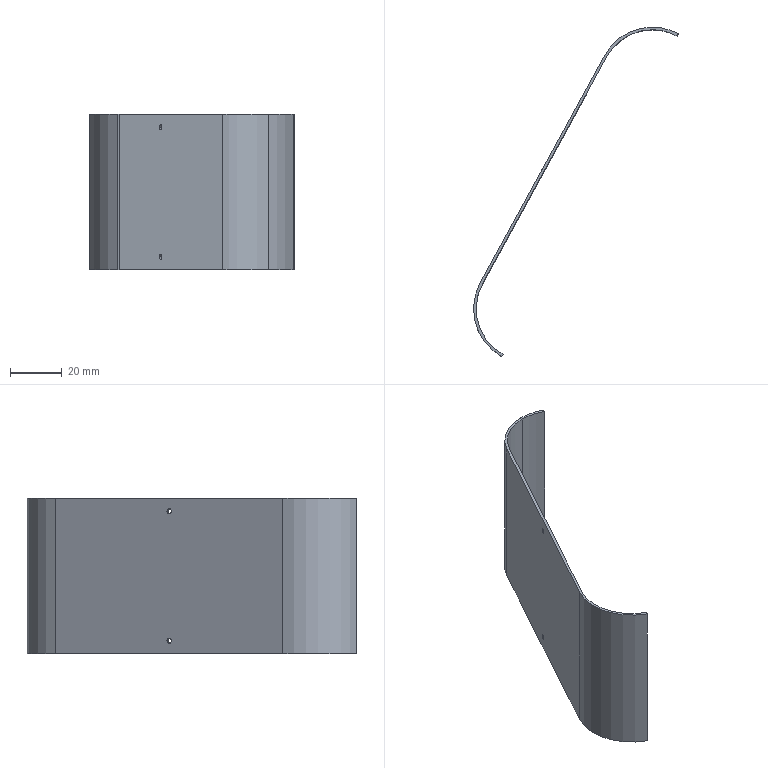Part | SolidWorks | features BaseBody 1 | 1 solid | 16 faces | box 79.069 x 127.155 x 60 mm | volume 9858 mm3 | cylinder 10 | plane 6 | commonest cylinder face diameters 2 x4 40 x3 42 x3
STEP:
#1=CARTESIAN_POINT('',(513.262,10.517,305.544));
#2=VERTEX_POINT('',#1);
#3=CARTESIAN_POINT('',(494.838,-0.4052,305.544));
#4=VERTEX_POINT('',#3);
#5=CARTESIAN_POINT('',(513.262,-10.483,305.544));
#6=DIRECTION('',(0.000000004,-0.000000009,1.));
#7=DIRECTION('',(0.,1.,0.000000009));
#8=AXIS2_PLACEMENT_3D('',#5,#6,#7);
#9=CIRCLE('',#8,21.);
#10=EDGE_CURVE('',#2,#4,#9,.T.);
#11=ORIENTED_EDGE('',*,*,#10,.F.);
#12=CARTESIAN_POINT('',(513.262,10.517,245.544));
#13=VERTEX_POINT('',#12);
#14=CARTESIAN_POINT('',(513.262,10.517,305.544));
#15=DIRECTION('',(-0.000000004,0.000000009,-1.));
#16=VECTOR('',#15,1000.);
#17=LINE('',#14,#16);
#18=EDGE_CURVE('',#2,#13,#17,.T.);
#19=ORIENTED_EDGE('',*,*,#18,.T.);
#20=CARTESIAN_POINT('',(494.838,-0.4052,245.544));
#21=VERTEX_POINT('',#20);
#22=CARTESIAN_POINT('',(513.262,-10.483,245.544));
#23=DIRECTION('',(-0.000000004,0.000000009,-1.));
#24=DIRECTION('',(0.,1.,0.000000009));
#25=AXIS2_PLACEMENT_3D('',#22,#23,#24);
#26=CIRCLE('',#25,21.);
#27=EDGE_CURVE('',#21,#13,#26,.T.);
#28=ORIENTED_EDGE('',*,*,#27,.F.);
#29=CARTESIAN_POINT('',(494.838,-0.4052,275.544));
#30=DIRECTION('',(-0.000000007,0.000000004,-1.));
#31=VECTOR('',#30,1000.);
#32=LINE('',#29,#31);
#33=EDGE_CURVE('',#4,#21,#32,.T.);
#34=ORIENTED_EDGE('',*,*,#33,.F.);
#35=EDGE_LOOP('',(#11,#19,#28,#34));
#36=FACE_OUTER_BOUND('',#35,.T.);
#37=CARTESIAN_POINT('',(513.262,-10.483,305.544));
#38=DIRECTION('',(-0.000000004,0.000000009,-1.));
#39=DIRECTION('',(0.,1.,0.000000009));
#40=AXIS2_PLACEMENT_3D('',#37,#38,#39);
#41=CYLINDRICAL_SURFACE('',#40,21.);
#42=ADVANCED_FACE('',(#36),#41,.T.);
#43=CARTESIAN_POINT('',(472.199,-43.874,300.544));
#44=VERTEX_POINT('',#43);
#45=CARTESIAN_POINT('',(471.24,-45.628,300.544));
#46=VERTEX_POINT('',#45);
#47=CARTESIAN_POINT('',(471.72,-44.751,300.544));
#48=DIRECTION('',(-0.8773,0.4799,0.000000008));
#49=DIRECTION('',(-0.4799,-0.8773,0.));
#50=AXIS2_PLACEMENT_3D('',#47,#48,#49);
#51=CIRCLE('',#50,1.);
#52=EDGE_CURVE('',#44,#46,#51,.T.);
#53=ORIENTED_EDGE('',*,*,#52,.F.);
#54=CARTESIAN_POINT('',(471.322,-43.394,300.544));
#55=VERTEX_POINT('',#54);
#56=CARTESIAN_POINT('',(471.313,-43.389,300.544));
#57=DIRECTION('',(-0.8773,0.4799,0.000000008));
#58=VECTOR('',#57,1000.);
#59=LINE('',#56,#58);
#60=EDGE_CURVE('',#44,#55,#59,.T.);
#61=ORIENTED_EDGE('',*,*,#60,.T.);
#62=CARTESIAN_POINT('',(470.362,-45.148,300.544));
#63=VERTEX_POINT('',#62);
#64=CARTESIAN_POINT('',(470.842,-44.271,300.544));
#65=DIRECTION('',(0.8773,-0.4799,-0.000000008));
#66=DIRECTION('',(-0.4799,-0.8773,0.));
#67=AXIS2_PLACEMENT_3D('',#64,#65,#66);
#68=CIRCLE('',#67,1.);
#69=EDGE_CURVE('',#63,#55,#68,.T.);
#70=ORIENTED_EDGE('',*,*,#69,.F.);
#71=CARTESIAN_POINT('',(470.354,-45.144,300.544));
#72=DIRECTION('',(-0.8773,0.4799,0.000000008));
#73=VECTOR('',#72,1000.);
#74=LINE('',#71,#73);
#75=EDGE_CURVE('',#46,#63,#74,.T.);
#76=ORIENTED_EDGE('',*,*,#75,.F.);
#77=EDGE_LOOP('',(#53,#61,#70,#76));
#78=FACE_OUTER_BOUND('',#77,.T.);
#79=CARTESIAN_POINT('',(470.833,-44.266,300.544));
#80=DIRECTION('',(-0.8773,0.4799,0.000000008));
#81=DIRECTION('',(-0.4799,-0.8773,0.));
#82=AXIS2_PLACEMENT_3D('',#79,#80,#81);
#83=CYLINDRICAL_SURFACE('',#82,1.);
#84=ADVANCED_FACE('',(#78),#83,.F.);
#85=CARTESIAN_POINT('',(472.199,-43.874,250.544));
#86=VERTEX_POINT('',#85);
#87=CARTESIAN_POINT('',(471.24,-45.628,250.544));
#88=VERTEX_POINT('',#87);
#89=CARTESIAN_POINT('',(471.72,-44.751,250.544));
#90=DIRECTION('',(-0.8773,0.4799,0.000000008));
#91=DIRECTION('',(-0.4799,-0.8773,0.));
#92=AXIS2_PLACEMENT_3D('',#89,#90,#91);
#93=CIRCLE('',#92,1.);
#94=EDGE_CURVE('',#86,#88,#93,.T.);
#95=ORIENTED_EDGE('',*,*,#94,.F.);
#96=CARTESIAN_POINT('',(471.322,-43.394,250.544));
#97=VERTEX_POINT('',#96);
#98=CARTESIAN_POINT('',(471.313,-43.389,250.544));
#99=DIRECTION('',(-0.8773,0.4799,0.000000008));
#100=VECTOR('',#99,1000.);
#101=LINE('',#98,#100);
#102=EDGE_CURVE('',#86,#97,#101,.T.);
#103=ORIENTED_EDGE('',*,*,#102,.T.);
#104=CARTESIAN_POINT('',(470.362,-45.148,250.544));
#105=VERTEX_POINT('',#104);
#106=CARTESIAN_POINT('',(470.842,-44.271,250.544));
#107=DIRECTION('',(0.8773,-0.4799,-0.000000008));
#108=DIRECTION('',(-0.4799,-0.8773,0.));
#109=AXIS2_PLACEMENT_3D('',#106,#107,#108);
#110=CIRCLE('',#109,1.);
#111=EDGE_CURVE('',#105,#97,#110,.T.);
#112=ORIENTED_EDGE('',*,*,#111,.F.);
#113=CARTESIAN_POINT('',(470.354,-45.144,250.544));
#114=DIRECTION('',(-0.8773,0.4799,0.000000008));
#115=VECTOR('',#114,1000.);
#116=LINE('',#113,#115);
#117=EDGE_CURVE('',#88,#105,#116,.T.);
#118=ORIENTED_EDGE('',*,*,#117,.F.);
#119=EDGE_LOOP('',(#95,#103,#112,#118));
#120=FACE_OUTER_BOUND('',#119,.T.);
#121=CARTESIAN_POINT('',(470.833,-44.266,250.544));
#122=DIRECTION('',(-0.8773,0.4799,0.000000008));
#123=DIRECTION('',(-0.4799,-0.8773,0.));
#124=AXIS2_PLACEMENT_3D('',#121,#122,#123);
#125=CYLINDRICAL_SURFACE('',#124,1.);
#126=ADVANCED_FACE('',(#120),#125,.F.);
#127=CARTESIAN_POINT('',(513.262,9.517,305.544));
#128=VERTEX_POINT('',#127);
#129=CARTESIAN_POINT('',(522.86,7.063,305.544));
#130=VERTEX_POINT('',#129);
#131=CARTESIAN_POINT('',(513.262,-10.483,305.544));
#132=DIRECTION('',(-0.000000004,0.000000009,-1.));
#133=DIRECTION('',(0.,1.,0.000000009));
#134=AXIS2_PLACEMENT_3D('',#131,#132,#133);
#135=CIRCLE('',#134,20.);
#136=EDGE_CURVE('',#128,#130,#135,.T.);
#137=ORIENTED_EDGE('',*,*,#136,.F.);
#138=CARTESIAN_POINT('',(513.262,9.517,245.544));
#139=VERTEX_POINT('',#138);
#140=CARTESIAN_POINT('',(513.262,9.517,305.544));
#141=DIRECTION('',(-0.000000004,0.000000009,-1.));
#142=VECTOR('',#141,1000.);
#143=LINE('',#140,#142);
#144=EDGE_CURVE('',#128,#139,#143,.T.);
#145=ORIENTED_EDGE('',*,*,#144,.T.);
#146=CARTESIAN_POINT('',(522.86,7.063,245.544));
#147=VERTEX_POINT('',#146);
#148=CARTESIAN_POINT('',(513.262,-10.483,245.544));
#149=DIRECTION('',(0.000000004,-0.000000009,1.));
#150=DIRECTION('',(0.,1.,0.000000009));
#151=AXIS2_PLACEMENT_3D('',#148,#149,#150);
#152=CIRCLE('',#151,20.);
#153=EDGE_CURVE('',#147,#139,#152,.T.);
#154=ORIENTED_EDGE('',*,*,#153,.F.);
#155=CARTESIAN_POINT('',(522.86,7.063,305.544));
#156=DIRECTION('',(-0.000000004,0.000000009,-1.));
#157=VECTOR('',#156,1000.);
#158=LINE('',#155,#157);
#159=EDGE_CURVE('',#130,#147,#158,.T.);
#160=ORIENTED_EDGE('',*,*,#159,.F.);
#161=EDGE_LOOP('',(#137,#145,#154,#160));
#162=FACE_OUTER_BOUND('',#161,.T.);
#163=CARTESIAN_POINT('',(513.262,-10.483,305.544));
#164=DIRECTION('',(-0.000000004,0.000000009,-1.));
#165=DIRECTION('',(0.,1.,0.000000009));
#166=AXIS2_PLACEMENT_3D('',#163,#164,#165);
#167=CYLINDRICAL_SURFACE('',#166,20.);
#168=ADVANCED_FACE('',(#162),#167,.F.);
#169=CARTESIAN_POINT('',(446.847,-88.137,245.544));
#170=VERTEX_POINT('',#169);
#171=CARTESIAN_POINT('',(446.847,-88.137,305.544));
#172=VERTEX_POINT('',#171);
#173=CARTESIAN_POINT('',(446.847,-88.137,275.544));
#174=DIRECTION('',(0.000000007,-0.000000004,1.));
#175=VECTOR('',#174,1000.);
#176=LINE('',#173,#175);
#177=EDGE_CURVE('',#170,#172,#176,.T.);
#178=ORIENTED_EDGE('',*,*,#177,.T.);
#179=CARTESIAN_POINT('',(470.842,-44.271,305.544));
#180=DIRECTION('',(0.4799,0.8773,0.));
#181=VECTOR('',#180,1000.);
#182=LINE('',#179,#181);
#183=EDGE_CURVE('',#172,#4,#182,.T.);
#184=ORIENTED_EDGE('',*,*,#183,.T.);
#185=ORIENTED_EDGE('',*,*,#33,.T.);
#186=CARTESIAN_POINT('',(470.842,-44.271,245.544));
#187=DIRECTION('',(-0.4799,-0.8773,0.));
#188=VECTOR('',#187,1000.);
#189=LINE('',#186,#188);
#190=EDGE_CURVE('',#21,#170,#189,.T.);
#191=ORIENTED_EDGE('',*,*,#190,.T.);
#192=EDGE_LOOP('',(#178,#184,#185,#191));
#193=FACE_OUTER_BOUND('',#192,.T.);
#194=ORIENTED_EDGE('',*,*,#69,.T.);
#195=CARTESIAN_POINT('',(470.842,-44.271,300.544));
#196=DIRECTION('',(0.8773,-0.4799,-0.000000008));
#197=DIRECTION('',(-0.4799,-0.8773,0.));
#198=AXIS2_PLACEMENT_3D('',#195,#196,#197);
#199=CIRCLE('',#198,1.);
#200=EDGE_CURVE('',#55,#63,#199,.T.);
#201=ORIENTED_EDGE('',*,*,#200,.T.);
#202=EDGE_LOOP('',(#194,#201));
#203=FACE_BOUND('',#202,.T.);
#204=ORIENTED_EDGE('',*,*,#111,.T.);
#205=CARTESIAN_POINT('',(470.842,-44.271,250.544));
#206=DIRECTION('',(0.8773,-0.4799,-0.000000008));
#207=DIRECTION('',(-0.4799,-0.8773,0.));
#208=AXIS2_PLACEMENT_3D('',#205,#206,#207);
#209=CIRCLE('',#208,1.);
#210=EDGE_CURVE('',#97,#105,#209,.T.);
#211=ORIENTED_EDGE('',*,*,#210,.T.);
#212=EDGE_LOOP('',(#204,#211));
#213=FACE_BOUND('',#212,.T.);
#214=CARTESIAN_POINT('',(470.842,-44.271,275.544));
#215=DIRECTION('',(-0.8773,0.4799,0.000000008));
#216=DIRECTION('',(-0.4799,-0.8773,0.));
#217=AXIS2_PLACEMENT_3D('',#214,#215,#216);
#218=PLANE('',#217);
#219=ADVANCED_FACE('',(#193,#203,#213),#218,.T.);
#220=CARTESIAN_POINT('',(523.34,7.94,305.544));
#221=VERTEX_POINT('',#220);
#222=CARTESIAN_POINT('',(522.86,7.063,305.544));
#223=DIRECTION('',(-0.4799,-0.8773,0.));
#224=VECTOR('',#223,1000.);
#225=LINE('',#222,#224);
#226=EDGE_CURVE('',#221,#130,#225,.T.);
#227=ORIENTED_EDGE('',*,*,#226,.F.);
#228=CARTESIAN_POINT('',(513.262,-10.483,305.544));
#229=DIRECTION('',(0.000000004,-0.000000009,1.));
#230=DIRECTION('',(0.,1.,0.000000009));
#231=AXIS2_PLACEMENT_3D('',#228,#229,#230);
#232=CIRCLE('',#231,21.);
#233=EDGE_CURVE('',#221,#2,#232,.T.);
#234=ORIENTED_EDGE('',*,*,#233,.T.);
#235=ORIENTED_EDGE('',*,*,#10,.T.);
#236=ORIENTED_EDGE('',*,*,#183,.F.);
#237=CARTESIAN_POINT('',(455.192,-116.639,305.544));
#238=VERTEX_POINT('',#237);
#239=CARTESIAN_POINT('',(465.27,-98.215,305.544));
#240=DIRECTION('',(0.000000004,-0.000000009,1.));
#241=DIRECTION('',(0.,-1.,-0.000000009));
#242=AXIS2_PLACEMENT_3D('',#239,#240,#241);
#243=CIRCLE('',#242,21.);
#244=EDGE_CURVE('',#172,#238,#243,.T.);
#245=ORIENTED_EDGE('',*,*,#244,.T.);
#246=CARTESIAN_POINT('',(455.672,-115.761,305.544));
#247=VERTEX_POINT('',#246);
#248=CARTESIAN_POINT('',(455.672,-115.761,305.544));
#249=DIRECTION('',(-0.4799,-0.8773,0.));
#250=VECTOR('',#249,1000.);
#251=LINE('',#248,#250);
#252=EDGE_CURVE('',#247,#238,#251,.T.);
#253=ORIENTED_EDGE('',*,*,#252,.F.);
#254=CARTESIAN_POINT('',(447.724,-88.617,305.544));
#255=VERTEX_POINT('',#254);
#256=CARTESIAN_POINT('',(465.27,-98.215,305.544));
#257=DIRECTION('',(-0.000000004,0.000000009,-1.));
#258=DIRECTION('',(0.,-1.,-0.000000009));
#259=AXIS2_PLACEMENT_3D('',#256,#257,#258);
#260=CIRCLE('',#259,20.);
#261=EDGE_CURVE('',#247,#255,#260,.T.);
#262=ORIENTED_EDGE('',*,*,#261,.T.);
#263=CARTESIAN_POINT('',(495.715,-0.8851,305.544));
#264=VERTEX_POINT('',#263);
#265=CARTESIAN_POINT('',(447.724,-88.617,305.544));
#266=DIRECTION('',(0.4799,0.8773,0.000000006));
#267=VECTOR('',#266,1000.);
#268=LINE('',#265,#267);
#269=EDGE_CURVE('',#255,#264,#268,.T.);
#270=ORIENTED_EDGE('',*,*,#269,.T.);
#271=CARTESIAN_POINT('',(513.262,-10.483,305.544));
#272=DIRECTION('',(-0.000000004,0.000000009,-1.));
#273=DIRECTION('',(0.,1.,0.000000009));
#274=AXIS2_PLACEMENT_3D('',#271,#272,#273);
#275=CIRCLE('',#274,20.);
#276=EDGE_CURVE('',#264,#128,#275,.T.);
#277=ORIENTED_EDGE('',*,*,#276,.T.);
#278=ORIENTED_EDGE('',*,*,#136,.T.);
#279=EDGE_LOOP('',(#227,#234,#235,#236,#245,#253,#262,#270,#277,#278));
#280=FACE_OUTER_BOUND('',#279,.T.);
#281=CARTESIAN_POINT('',(505.313,16.661,305.544));
#282=DIRECTION('',(0.000000004,-0.000000009,1.));
#283=DIRECTION('',(0.,-1.,-0.000000009));
#284=AXIS2_PLACEMENT_3D('',#281,#282,#283);
#285=PLANE('',#284);
#286=ADVANCED_FACE('',(#280),#285,.T.);
#287=CARTESIAN_POINT('',(455.192,-116.639,245.544));
#288=VERTEX_POINT('',#287);
#289=CARTESIAN_POINT('',(465.27,-98.215,245.544));
#290=DIRECTION('',(0.000000004,-0.000000009,1.));
#291=DIRECTION('',(0.,-1.,-0.000000009));
#292=AXIS2_PLACEMENT_3D('',#289,#290,#291);
#293=CIRCLE('',#292,21.);
#294=EDGE_CURVE('',#170,#288,#293,.T.);
#295=ORIENTED_EDGE('',*,*,#294,.T.);
#296=CARTESIAN_POINT('',(455.192,-116.639,245.544));
#297=DIRECTION('',(0.000000004,-0.000000009,1.));
#298=VECTOR('',#297,1000.);
#299=LINE('',#296,#298);
#300=EDGE_CURVE('',#288,#238,#299,.T.);
#301=ORIENTED_EDGE('',*,*,#300,.T.);
#302=ORIENTED_EDGE('',*,*,#244,.F.);
#303=ORIENTED_EDGE('',*,*,#177,.F.);
#304=EDGE_LOOP('',(#295,#301,#302,#303));
#305=FACE_OUTER_BOUND('',#304,.T.);
#306=CARTESIAN_POINT('',(465.27,-98.215,245.544));
#307=DIRECTION('',(0.000000004,-0.000000009,1.));
#308=DIRECTION('',(0.,-1.,-0.000000009));
#309=AXIS2_PLACEMENT_3D('',#306,#307,#308);
#310=CYLINDRICAL_SURFACE('',#309,21.);
#311=ADVANCED_FACE('',(#305),#310,.T.);
#312=CARTESIAN_POINT('',(523.34,7.94,245.544));
#313=VERTEX_POINT('',#312);
#314=CARTESIAN_POINT('',(522.86,7.063,245.544));
#315=DIRECTION('',(0.4799,0.8773,0.));
#316=VECTOR('',#315,1000.);
#317=LINE('',#314,#316);
#318=EDGE_CURVE('',#147,#313,#317,.T.);
#319=ORIENTED_EDGE('',*,*,#318,.F.);
#320=ORIENTED_EDGE('',*,*,#153,.T.);
#321=CARTESIAN_POINT('',(495.715,-0.8851,245.544));
#322=VERTEX_POINT('',#321);
#323=CARTESIAN_POINT('',(513.262,-10.483,245.544));
#324=DIRECTION('',(0.000000004,-0.000000009,1.));
#325=DIRECTION('',(0.,1.,0.000000009));
#326=AXIS2_PLACEMENT_3D('',#323,#324,#325);
#327=CIRCLE('',#326,20.);
#328=EDGE_CURVE('',#139,#322,#327,.T.);
#329=ORIENTED_EDGE('',*,*,#328,.T.);
#330=CARTESIAN_POINT('',(447.724,-88.617,245.544));
#331=VERTEX_POINT('',#330);
#332=CARTESIAN_POINT('',(495.715,-0.8851,245.544));
#333=DIRECTION('',(-0.4799,-0.8773,-0.000000006));
#334=VECTOR('',#333,1000.);
#335=LINE('',#332,#334);
#336=EDGE_CURVE('',#322,#331,#335,.T.);
#337=ORIENTED_EDGE('',*,*,#336,.T.);
#338=CARTESIAN_POINT('',(455.672,-115.761,245.544));
#339=VERTEX_POINT('',#338);
#340=CARTESIAN_POINT('',(465.27,-98.215,245.544));
#341=DIRECTION('',(0.000000004,-0.000000009,1.));
#342=DIRECTION('',(0.,-1.,-0.000000009));
#343=AXIS2_PLACEMENT_3D('',#340,#341,#342);
#344=CIRCLE('',#343,20.);
#345=EDGE_CURVE('',#331,#339,#344,.T.);
#346=ORIENTED_EDGE('',*,*,#345,.T.);
#347=CARTESIAN_POINT('',(455.672,-115.761,245.544));
#348=DIRECTION('',(-0.4799,-0.8773,-0.000000006));
#349=VECTOR('',#348,1000.);
#350=LINE('',#347,#349);
#351=EDGE_CURVE('',#339,#288,#350,.T.);
#352=ORIENTED_EDGE('',*,*,#351,.T.);
#353=ORIENTED_EDGE('',*,*,#294,.F.);
#354=ORIENTED_EDGE('',*,*,#190,.F.);
#355=ORIENTED_EDGE('',*,*,#27,.T.);
#356=CARTESIAN_POINT('',(513.262,-10.483,245.544));
#357=DIRECTION('',(-0.000000004,0.000000009,-1.));
#358=DIRECTION('',(0.,1.,0.000000009));
#359=AXIS2_PLACEMENT_3D('',#356,#357,#358);
#360=CIRCLE('',#359,21.);
#361=EDGE_CURVE('',#13,#313,#360,.T.);
#362=ORIENTED_EDGE('',*,*,#361,.T.);
#363=EDGE_LOOP('',(#319,#320,#329,#337,#346,#352,#353,#354,#355,#362));
#364=FACE_OUTER_BOUND('',#363,.T.);
#365=CARTESIAN_POINT('',(438.126,-106.163,245.544));
#366=DIRECTION('',(-0.000000004,0.000000009,-1.));
#367=DIRECTION('',(0.,1.,0.000000009));
#368=AXIS2_PLACEMENT_3D('',#365,#366,#367);
#369=PLANE('',#368);
#370=ADVANCED_FACE('',(#364),#369,.T.);
#371=ORIENTED_EDGE('',*,*,#18,.F.);
#372=ORIENTED_EDGE('',*,*,#233,.F.);
#373=CARTESIAN_POINT('',(523.34,7.94,305.544));
#374=DIRECTION('',(-0.000000004,0.000000009,-1.));
#375=VECTOR('',#374,1000.);
#376=LINE('',#373,#375);
#377=EDGE_CURVE('',#221,#313,#376,.T.);
#378=ORIENTED_EDGE('',*,*,#377,.T.);
#379=ORIENTED_EDGE('',*,*,#361,.F.);
#380=EDGE_LOOP('',(#371,#372,#378,#379));
#381=FACE_OUTER_BOUND('',#380,.T.);
#382=CARTESIAN_POINT('',(513.262,-10.483,305.544));
#383=DIRECTION('',(-0.000000004,0.000000009,-1.));
#384=DIRECTION('',(0.,1.,0.000000009));
#385=AXIS2_PLACEMENT_3D('',#382,#383,#384);
#386=CYLINDRICAL_SURFACE('',#385,21.);
#387=ADVANCED_FACE('',(#381),#386,.T.);
#388=ORIENTED_EDGE('',*,*,#60,.F.);
#389=CARTESIAN_POINT('',(471.72,-44.751,300.544));
#390=DIRECTION('',(-0.8773,0.4799,0.000000008));
#391=DIRECTION('',(-0.4799,-0.8773,0.));
#392=AXIS2_PLACEMENT_3D('',#389,#390,#391);
#393=CIRCLE('',#392,1.);
#394=EDGE_CURVE('',#46,#44,#393,.T.);
#395=ORIENTED_EDGE('',*,*,#394,.F.);
#396=ORIENTED_EDGE('',*,*,#75,.T.);
#397=ORIENTED_EDGE('',*,*,#200,.F.);
#398=EDGE_LOOP('',(#388,#395,#396,#397));
#399=FACE_OUTER_BOUND('',#398,.T.);
#400=CARTESIAN_POINT('',(470.833,-44.266,300.544));
#401=DIRECTION('',(-0.8773,0.4799,0.000000008));
#402=DIRECTION('',(-0.4799,-0.8773,0.));
#403=AXIS2_PLACEMENT_3D('',#400,#401,#402);
#404=CYLINDRICAL_SURFACE('',#403,1.);
#405=ADVANCED_FACE('',(#399),#404,.F.);
#406=ORIENTED_EDGE('',*,*,#102,.F.);
#407=CARTESIAN_POINT('',(471.72,-44.751,250.544));
#408=DIRECTION('',(-0.8773,0.4799,0.000000008));
#409=DIRECTION('',(-0.4799,-0.8773,0.));
#410=AXIS2_PLACEMENT_3D('',#407,#408,#409);
#411=CIRCLE('',#410,1.);
#412=EDGE_CURVE('',#88,#86,#411,.T.);
#413=ORIENTED_EDGE('',*,*,#412,.F.);
#414=ORIENTED_EDGE('',*,*,#117,.T.);
#415=ORIENTED_EDGE('',*,*,#210,.F.);
#416=EDGE_LOOP('',(#406,#413,#414,#415));
#417=FACE_OUTER_BOUND('',#416,.T.);
#418=CARTESIAN_POINT('',(470.833,-44.266,250.544));
#419=DIRECTION('',(-0.8773,0.4799,0.000000008));
#420=DIRECTION('',(-0.4799,-0.8773,0.));
#421=AXIS2_PLACEMENT_3D('',#418,#419,#420);
#422=CYLINDRICAL_SURFACE('',#421,1.);
#423=ADVANCED_FACE('',(#417),#422,.F.);
#424=ORIENTED_EDGE('',*,*,#144,.F.);
#425=ORIENTED_EDGE('',*,*,#276,.F.);
#426=CARTESIAN_POINT('',(495.715,-0.8851,305.544));
#427=DIRECTION('',(0.000000004,-0.000000009,1.));
#428=VECTOR('',#427,1000.);
#429=LINE('',#426,#428);
#430=EDGE_CURVE('',#322,#264,#429,.T.);
#431=ORIENTED_EDGE('',*,*,#430,.F.);
#432=ORIENTED_EDGE('',*,*,#328,.F.);
#433=EDGE_LOOP('',(#424,#425,#431,#432));
#434=FACE_OUTER_BOUND('',#433,.T.);
#435=CARTESIAN_POINT('',(513.262,-10.483,305.544));
#436=DIRECTION('',(-0.000000004,0.000000009,-1.));
#437=DIRECTION('',(0.,1.,0.000000009));
#438=AXIS2_PLACEMENT_3D('',#435,#436,#437);
#439=CYLINDRICAL_SURFACE('',#438,20.);
#440=ADVANCED_FACE('',(#434),#439,.F.);
#441=ORIENTED_EDGE('',*,*,#269,.F.);
#442=CARTESIAN_POINT('',(447.724,-88.617,275.544));
#443=DIRECTION('',(0.000000007,-0.000000004,1.));
#444=VECTOR('',#443,1000.);
#445=LINE('',#442,#444);
#446=EDGE_CURVE('',#331,#255,#445,.T.);
#447=ORIENTED_EDGE('',*,*,#446,.F.);
#448=ORIENTED_EDGE('',*,*,#336,.F.);
#449=ORIENTED_EDGE('',*,*,#430,.T.);
#450=EDGE_LOOP('',(#441,#447,#448,#449));
#451=FACE_OUTER_BOUND('',#450,.T.);
#452=ORIENTED_EDGE('',*,*,#394,.T.);
#453=ORIENTED_EDGE('',*,*,#52,.T.);
#454=EDGE_LOOP('',(#452,#453));
#455=FACE_BOUND('',#454,.T.);
#456=ORIENTED_EDGE('',*,*,#412,.T.);
#457=ORIENTED_EDGE('',*,*,#94,.T.);
#458=EDGE_LOOP('',(#456,#457));
#459=FACE_BOUND('',#458,.T.);
#460=CARTESIAN_POINT('',(471.72,-44.751,275.544));
#461=DIRECTION('',(-0.8773,0.4799,0.000000008));
#462=DIRECTION('',(-0.4799,-0.8773,0.));
#463=AXIS2_PLACEMENT_3D('',#460,#461,#462);
#464=PLANE('',#463);
#465=ADVANCED_FACE('',(#451,#455,#459),#464,.F.);
#466=CARTESIAN_POINT('',(455.672,-115.761,245.544));
#467=DIRECTION('',(0.000000004,-0.000000009,1.));
#468=VECTOR('',#467,1000.);
#469=LINE('',#466,#468);
#470=EDGE_CURVE('',#339,#247,#469,.T.);
#471=ORIENTED_EDGE('',*,*,#470,.F.);
#472=ORIENTED_EDGE('',*,*,#345,.F.);
#473=ORIENTED_EDGE('',*,*,#446,.T.);
#474=ORIENTED_EDGE('',*,*,#261,.F.);
#475=EDGE_LOOP('',(#471,#472,#473,#474));
#476=FACE_OUTER_BOUND('',#475,.T.);
#477=CARTESIAN_POINT('',(465.27,-98.215,245.544));
#478=DIRECTION('',(0.000000004,-0.000000009,1.));
#479=DIRECTION('',(0.,-1.,-0.000000009));
#480=AXIS2_PLACEMENT_3D('',#477,#478,#479);
#481=CYLINDRICAL_SURFACE('',#480,20.);
#482=ADVANCED_FACE('',(#476),#481,.F.);
#483=ORIENTED_EDGE('',*,*,#351,.F.);
#484=ORIENTED_EDGE('',*,*,#470,.T.);
#485=ORIENTED_EDGE('',*,*,#252,.T.);
#486=ORIENTED_EDGE('',*,*,#300,.F.);
#487=EDGE_LOOP('',(#483,#484,#485,#486));
#488=FACE_OUTER_BOUND('',#487,.T.);
#489=CARTESIAN_POINT('',(455.672,-115.761,245.544));
#490=DIRECTION('',(0.8773,-0.4799,-0.000000008));
#491=DIRECTION('',(0.4799,0.8773,0.));
#492=AXIS2_PLACEMENT_3D('',#489,#490,#491);
#493=PLANE('',#492);
#494=ADVANCED_FACE('',(#488),#493,.T.);
#495=ORIENTED_EDGE('',*,*,#226,.T.);
#496=ORIENTED_EDGE('',*,*,#159,.T.);
#497=ORIENTED_EDGE('',*,*,#318,.T.);
#498=ORIENTED_EDGE('',*,*,#377,.F.);
#499=EDGE_LOOP('',(#495,#496,#497,#498));
#500=FACE_OUTER_BOUND('',#499,.T.);
#501=CARTESIAN_POINT('',(522.86,7.063,305.544));
#502=DIRECTION('',(0.8773,-0.4799,-0.000000008));
#503=DIRECTION('',(0.4799,0.8773,0.));
#504=AXIS2_PLACEMENT_3D('',#501,#502,#503);
#505=PLANE('',#504);
#506=ADVANCED_FACE('',(#500),#505,.T.);
#507=CLOSED_SHELL('',(#42,#84,#126,#168,#219,#286,#311,#370,#387,#405,#423,#440,#465,#482,#494,#506));
#508=MANIFOLD_SOLID_BREP('',#507);
#509=CARTESIAN_POINT('',(0.,0.,0.));
#510=DIRECTION('',(0.,0.,1.));
#511=DIRECTION('',(1.,0.,0.));
#512=AXIS2_PLACEMENT_3D('',#509,#510,#511);
#513=(LENGTH_UNIT()NAMED_UNIT(*)SI_UNIT(.MILLI.,.METRE.));
#514=UNCERTAINTY_MEASURE_WITH_UNIT(LENGTH_MEASURE(0.00001),#513,'','');
#515=(NAMED_UNIT(*)PLANE_ANGLE_UNIT()SI_UNIT($,.RADIAN.));
#516=(NAMED_UNIT(*)SI_UNIT($,.STERADIAN.)SOLID_ANGLE_UNIT());
#517=(GEOMETRIC_REPRESENTATION_CONTEXT(3)GLOBAL_UNCERTAINTY_ASSIGNED_CONTEXT((#514))GLOBAL_UNIT_ASSIGNED_CONTEXT((#513,#515,#516))REPRESENTATION_CONTEXT('',''));
#518=ADVANCED_BREP_SHAPE_REPRESENTATION('',(#508,#512),#517);